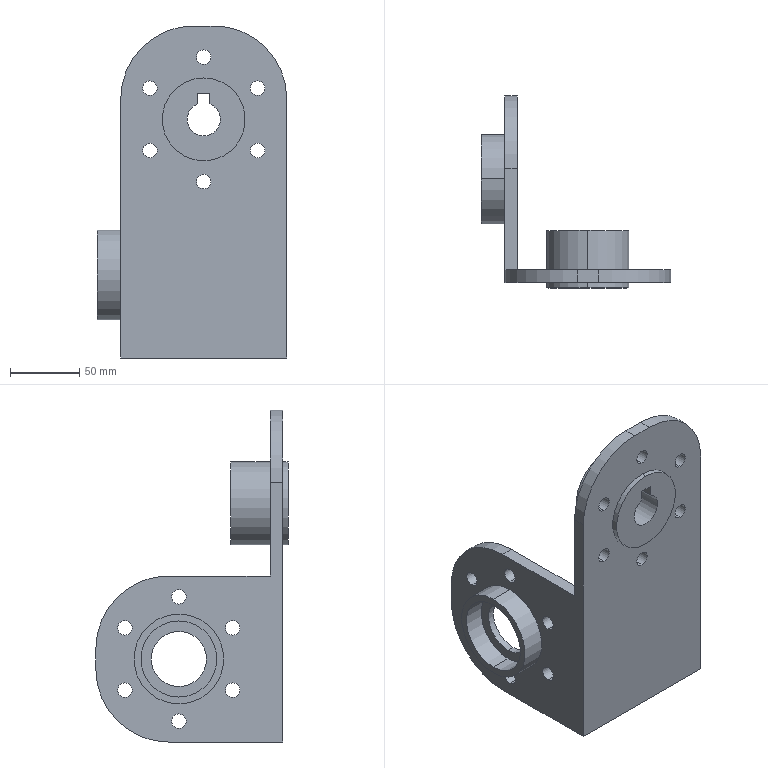Part | SolidWorks | features ICE 6, BaseBody 1, CirPattern 1 | 1 solid | 58 faces | box 137 x 139 x 240 mm | volume 432649 mm3 | cylinder 41 | plane 17 | commonest cylinder face diameters 10.5 x24 60 x6 105 x4 40 x2 55 x2 65 x2